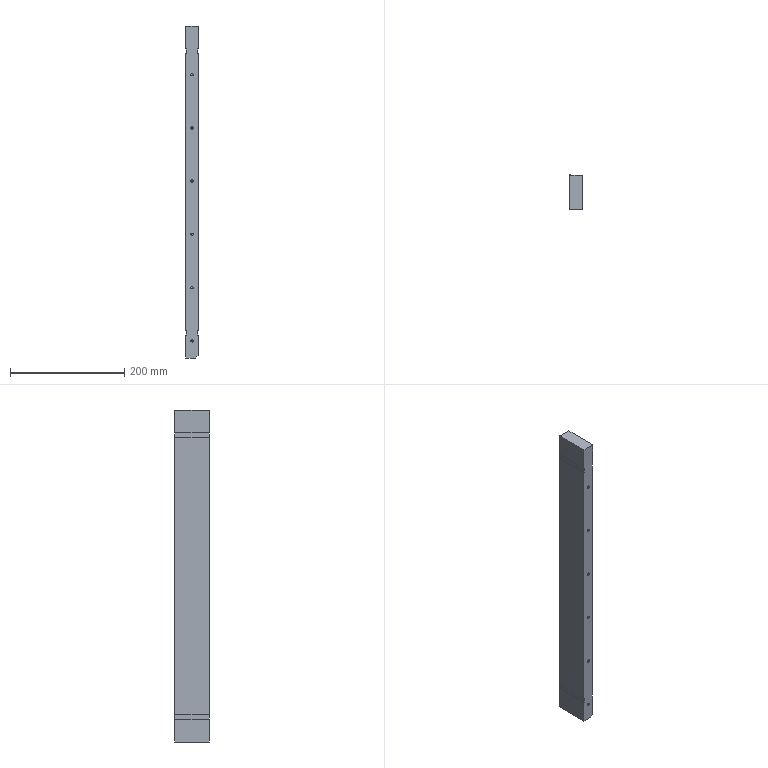Part | NX | features BREP 1 | 1 solid | 89 faces | box 22 x 61 x 580 mm | volume 749661 mm3 | cone 32 | cylinder 32 | plane 25 | commonest cylinder face diameters 4.2 x32